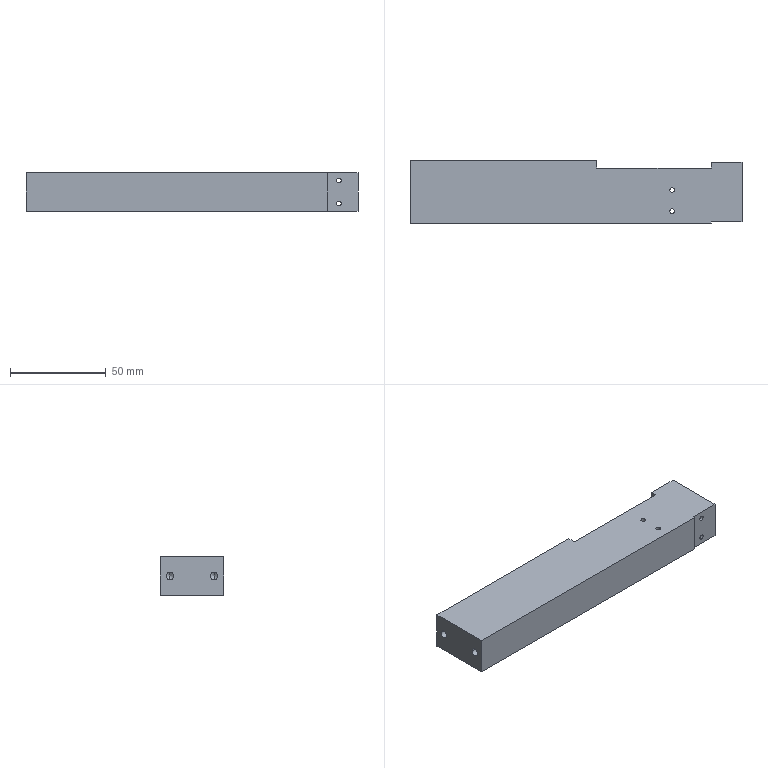Part | SolidWorks | features BaseBody 1 | 1 solid | 36 faces | box 173.5 x 33 x 20 mm | volume 108000 mm3 | cylinder 16 | plane 12 | cone 8 | commonest cylinder face diameters 2.459 x8 4.134 x8
STEP:
#1=CARTESIAN_POINT('',(21.865,283.98,0.));
#2=VERTEX_POINT('',#1);
#3=CARTESIAN_POINT('',(19.406,283.98,0.));
#4=VERTEX_POINT('',#3);
#5=CARTESIAN_POINT('',(20.636,283.98,0.));
#6=DIRECTION('',(0.,0.,-1.));
#7=DIRECTION('',(1.,0.,0.));
#8=AXIS2_PLACEMENT_3D('',#5,#6,#7);
#9=CIRCLE('',#8,1.23);
#10=EDGE_CURVE('',#2,#4,#9,.T.);
#11=ORIENTED_EDGE('',*,*,#10,.T.);
#12=CARTESIAN_POINT('',(19.406,283.98,20.));
#13=VERTEX_POINT('',#12);
#14=CARTESIAN_POINT('',(19.406,283.98,-157.739));
#15=DIRECTION('',(0.,0.,1.));
#16=VECTOR('',#15,1000.);
#17=LINE('',#14,#16);
#18=EDGE_CURVE('',#4,#13,#17,.T.);
#19=ORIENTED_EDGE('',*,*,#18,.T.);
#20=CARTESIAN_POINT('',(21.865,283.98,20.));
#21=VERTEX_POINT('',#20);
#22=CARTESIAN_POINT('',(20.636,283.98,20.));
#23=DIRECTION('',(0.,0.,-1.));
#24=DIRECTION('',(1.,0.,0.));
#25=AXIS2_PLACEMENT_3D('',#22,#23,#24);
#26=CIRCLE('',#25,1.23);
#27=EDGE_CURVE('',#21,#13,#26,.T.);
#28=ORIENTED_EDGE('',*,*,#27,.F.);
#29=CARTESIAN_POINT('',(21.865,283.98,-157.739));
#30=DIRECTION('',(0.,0.,1.));
#31=VECTOR('',#30,1000.);
#32=LINE('',#29,#31);
#33=EDGE_CURVE('',#2,#21,#32,.T.);
#34=ORIENTED_EDGE('',*,*,#33,.F.);
#35=EDGE_LOOP('',(#11,#19,#28,#34));
#36=FACE_OUTER_BOUND('',#35,.T.);
#37=CARTESIAN_POINT('',(20.636,283.98,-157.739));
#38=DIRECTION('',(0.,0.,1.));
#39=DIRECTION('',(1.,0.,0.));
#40=AXIS2_PLACEMENT_3D('',#37,#38,#39);
#41=CYLINDRICAL_SURFACE('',#40,1.23);
#42=ADVANCED_FACE('',(#36),#41,.F.);
#43=CARTESIAN_POINT('',(21.865,272.98,0.));
#44=VERTEX_POINT('',#43);
#45=CARTESIAN_POINT('',(19.406,272.98,0.));
#46=VERTEX_POINT('',#45);
#47=CARTESIAN_POINT('',(20.636,272.98,0.));
#48=DIRECTION('',(0.,0.,-1.));
#49=DIRECTION('',(1.,0.,0.));
#50=AXIS2_PLACEMENT_3D('',#47,#48,#49);
#51=CIRCLE('',#50,1.23);
#52=EDGE_CURVE('',#44,#46,#51,.T.);
#53=ORIENTED_EDGE('',*,*,#52,.T.);
#54=CARTESIAN_POINT('',(19.406,272.98,20.));
#55=VERTEX_POINT('',#54);
#56=CARTESIAN_POINT('',(19.406,272.98,-157.739));
#57=DIRECTION('',(0.,0.,1.));
#58=VECTOR('',#57,1000.);
#59=LINE('',#56,#58);
#60=EDGE_CURVE('',#46,#55,#59,.T.);
#61=ORIENTED_EDGE('',*,*,#60,.T.);
#62=CARTESIAN_POINT('',(21.865,272.98,20.));
#63=VERTEX_POINT('',#62);
#64=CARTESIAN_POINT('',(20.636,272.98,20.));
#65=DIRECTION('',(0.,0.,-1.));
#66=DIRECTION('',(1.,0.,0.));
#67=AXIS2_PLACEMENT_3D('',#64,#65,#66);
#68=CIRCLE('',#67,1.23);
#69=EDGE_CURVE('',#63,#55,#68,.T.);
#70=ORIENTED_EDGE('',*,*,#69,.F.);
#71=CARTESIAN_POINT('',(21.865,272.98,-157.739));
#72=DIRECTION('',(0.,0.,1.));
#73=VECTOR('',#72,1000.);
#74=LINE('',#71,#73);
#75=EDGE_CURVE('',#44,#63,#74,.T.);
#76=ORIENTED_EDGE('',*,*,#75,.F.);
#77=EDGE_LOOP('',(#53,#61,#70,#76));
#78=FACE_OUTER_BOUND('',#77,.T.);
#79=CARTESIAN_POINT('',(20.636,272.98,-157.739));
#80=DIRECTION('',(0.,0.,1.));
#81=DIRECTION('',(1.,0.,0.));
#82=AXIS2_PLACEMENT_3D('',#79,#80,#81);
#83=CYLINDRICAL_SURFACE('',#82,1.23);
#84=ADVANCED_FACE('',(#78),#83,.F.);
#85=CARTESIAN_POINT('',(-1.797,289.48,10.));
#86=VERTEX_POINT('',#85);
#87=CARTESIAN_POINT('',(-3.864,289.48,7.933));
#88=VERTEX_POINT('',#87);
#89=CARTESIAN_POINT('',(-3.864,289.48,10.));
#90=DIRECTION('',(0.,1.,0.));
#91=DIRECTION('',(-1.,0.,0.));
#92=AXIS2_PLACEMENT_3D('',#89,#90,#91);
#93=CIRCLE('',#92,2.067);
#94=EDGE_CURVE('',#86,#88,#93,.T.);
#95=ORIENTED_EDGE('',*,*,#94,.F.);
#96=CARTESIAN_POINT('',(-1.797,295.48,10.));
#97=VERTEX_POINT('',#96);
#98=CARTESIAN_POINT('',(-1.797,294.48,10.));
#99=DIRECTION('',(0.,1.,0.));
#100=VECTOR('',#99,1000.);
#101=LINE('',#98,#100);
#102=EDGE_CURVE('',#86,#97,#101,.T.);
#103=ORIENTED_EDGE('',*,*,#102,.T.);
#104=CARTESIAN_POINT('',(-5.931,295.48,10.));
#105=VERTEX_POINT('',#104);
#106=CARTESIAN_POINT('',(-3.864,295.48,10.));
#107=DIRECTION('',(0.,-1.,0.));
#108=DIRECTION('',(-1.,0.,0.));
#109=AXIS2_PLACEMENT_3D('',#106,#107,#108);
#110=CIRCLE('',#109,2.067);
#111=EDGE_CURVE('',#105,#97,#110,.T.);
#112=ORIENTED_EDGE('',*,*,#111,.F.);
#113=CARTESIAN_POINT('',(-5.931,289.48,10.));
#114=VERTEX_POINT('',#113);
#115=CARTESIAN_POINT('',(-5.931,294.48,10.));
#116=DIRECTION('',(0.,1.,0.));
#117=VECTOR('',#116,1000.);
#118=LINE('',#115,#117);
#119=EDGE_CURVE('',#114,#105,#118,.T.);
#120=ORIENTED_EDGE('',*,*,#119,.F.);
#121=CARTESIAN_POINT('',(-3.864,289.48,10.));
#122=DIRECTION('',(0.,1.,0.));
#123=DIRECTION('',(-1.,0.,0.));
#124=AXIS2_PLACEMENT_3D('',#121,#122,#123);
#125=CIRCLE('',#124,2.067);
#126=EDGE_CURVE('',#88,#114,#125,.T.);
#127=ORIENTED_EDGE('',*,*,#126,.F.);
#128=EDGE_LOOP('',(#95,#103,#112,#120,#127));
#129=FACE_OUTER_BOUND('',#128,.T.);
#130=CARTESIAN_POINT('',(-3.864,294.48,10.));
#131=DIRECTION('',(0.,1.,0.));
#132=DIRECTION('',(-1.,0.,0.));
#133=AXIS2_PLACEMENT_3D('',#130,#131,#132);
#134=CYLINDRICAL_SURFACE('',#133,2.067);
#135=ADVANCED_FACE('',(#129),#134,.F.);
#136=CARTESIAN_POINT('',(28.203,289.48,10.));
#137=VERTEX_POINT('',#136);
#138=CARTESIAN_POINT('',(26.136,289.48,7.933));
#139=VERTEX_POINT('',#138);
#140=CARTESIAN_POINT('',(26.136,289.48,10.));
#141=DIRECTION('',(0.,1.,0.));
#142=DIRECTION('',(-1.,0.,0.));
#143=AXIS2_PLACEMENT_3D('',#140,#141,#142);
#144=CIRCLE('',#143,2.067);
#145=EDGE_CURVE('',#137,#139,#144,.T.);
#146=ORIENTED_EDGE('',*,*,#145,.F.);
#147=CARTESIAN_POINT('',(28.203,295.48,10.));
#148=VERTEX_POINT('',#147);
#149=CARTESIAN_POINT('',(28.203,294.48,10.));
#150=DIRECTION('',(0.,1.,0.));
#151=VECTOR('',#150,1000.);
#152=LINE('',#149,#151);
#153=EDGE_CURVE('',#137,#148,#152,.T.);
#154=ORIENTED_EDGE('',*,*,#153,.T.);
#155=CARTESIAN_POINT('',(24.069,295.48,10.));
#156=VERTEX_POINT('',#155);
#157=CARTESIAN_POINT('',(26.136,295.48,10.));
#158=DIRECTION('',(0.,-1.,0.));
#159=DIRECTION('',(-1.,0.,0.));
#160=AXIS2_PLACEMENT_3D('',#157,#158,#159);
#161=CIRCLE('',#160,2.067);
#162=EDGE_CURVE('',#156,#148,#161,.T.);
#163=ORIENTED_EDGE('',*,*,#162,.F.);
#164=CARTESIAN_POINT('',(24.069,289.48,10.));
#165=VERTEX_POINT('',#164);
#166=CARTESIAN_POINT('',(24.069,294.48,10.));
#167=DIRECTION('',(0.,1.,0.));
#168=VECTOR('',#167,1000.);
#169=LINE('',#166,#168);
#170=EDGE_CURVE('',#165,#156,#169,.T.);
#171=ORIENTED_EDGE('',*,*,#170,.F.);
#172=CARTESIAN_POINT('',(26.136,289.48,10.));
#173=DIRECTION('',(0.,1.,0.));
#174=DIRECTION('',(-1.,0.,0.));
#175=AXIS2_PLACEMENT_3D('',#172,#173,#174);
#176=CIRCLE('',#175,2.067);
#177=EDGE_CURVE('',#139,#165,#176,.T.);
#178=ORIENTED_EDGE('',*,*,#177,.F.);
#179=EDGE_LOOP('',(#146,#154,#163,#171,#178));
#180=FACE_OUTER_BOUND('',#179,.T.);
#181=CARTESIAN_POINT('',(26.136,294.48,10.));
#182=DIRECTION('',(0.,1.,0.));
#183=DIRECTION('',(-1.,0.,0.));
#184=AXIS2_PLACEMENT_3D('',#181,#182,#183);
#185=CYLINDRICAL_SURFACE('',#184,2.067);
#186=ADVANCED_FACE('',(#180),#185,.F.);
#187=CARTESIAN_POINT('',(45.906,267.48,16.));
#188=VERTEX_POINT('',#187);
#189=CARTESIAN_POINT('',(48.365,267.48,16.));
#190=VERTEX_POINT('',#189);
#191=CARTESIAN_POINT('',(47.136,267.48,16.));
#192=DIRECTION('',(0.,-1.,0.));
#193=DIRECTION('',(-1.,0.,0.));
#194=AXIS2_PLACEMENT_3D('',#191,#192,#193);
#195=CIRCLE('',#194,1.23);
#196=EDGE_CURVE('',#188,#190,#195,.T.);
#197=ORIENTED_EDGE('',*,*,#196,.T.);
#198=CARTESIAN_POINT('',(48.365,298.48,16.));
#199=VERTEX_POINT('',#198);
#200=CARTESIAN_POINT('',(48.365,121.741,16.));
#201=DIRECTION('',(0.,1.,0.));
#202=VECTOR('',#201,1000.);
#203=LINE('',#200,#202);
#204=EDGE_CURVE('',#190,#199,#203,.T.);
#205=ORIENTED_EDGE('',*,*,#204,.T.);
#206=CARTESIAN_POINT('',(45.906,298.48,16.));
#207=VERTEX_POINT('',#206);
#208=CARTESIAN_POINT('',(47.136,298.48,16.));
#209=DIRECTION('',(0.,-1.,0.));
#210=DIRECTION('',(-1.,0.,0.));
#211=AXIS2_PLACEMENT_3D('',#208,#209,#210);
#212=CIRCLE('',#211,1.23);
#213=EDGE_CURVE('',#207,#199,#212,.T.);
#214=ORIENTED_EDGE('',*,*,#213,.F.);
#215=CARTESIAN_POINT('',(45.906,121.741,16.));
#216=DIRECTION('',(0.,1.,0.));
#217=VECTOR('',#216,1000.);
#218=LINE('',#215,#217);
#219=EDGE_CURVE('',#188,#207,#218,.T.);
#220=ORIENTED_EDGE('',*,*,#219,.F.);
#221=EDGE_LOOP('',(#197,#205,#214,#220));
#222=FACE_OUTER_BOUND('',#221,.T.);
#223=CARTESIAN_POINT('',(47.136,121.741,16.));
#224=DIRECTION('',(0.,1.,0.));
#225=DIRECTION('',(-1.,0.,0.));
#226=AXIS2_PLACEMENT_3D('',#223,#224,#225);
#227=CYLINDRICAL_SURFACE('',#226,1.23);
#228=ADVANCED_FACE('',(#222),#227,.F.);
#229=CARTESIAN_POINT('',(45.906,267.48,4.));
#230=VERTEX_POINT('',#229);
#231=CARTESIAN_POINT('',(48.365,267.48,4.));
#232=VERTEX_POINT('',#231);
#233=CARTESIAN_POINT('',(47.136,267.48,4.));
#234=DIRECTION('',(0.,-1.,0.));
#235=DIRECTION('',(-1.,0.,0.));
#236=AXIS2_PLACEMENT_3D('',#233,#234,#235);
#237=CIRCLE('',#236,1.23);
#238=EDGE_CURVE('',#230,#232,#237,.T.);
#239=ORIENTED_EDGE('',*,*,#238,.T.);
#240=CARTESIAN_POINT('',(48.365,298.48,4.));
#241=VERTEX_POINT('',#240);
#242=CARTESIAN_POINT('',(48.365,121.741,4.));
#243=DIRECTION('',(0.,1.,0.));
#244=VECTOR('',#243,1000.);
#245=LINE('',#242,#244);
#246=EDGE_CURVE('',#232,#241,#245,.T.);
#247=ORIENTED_EDGE('',*,*,#246,.T.);
#248=CARTESIAN_POINT('',(45.906,298.48,4.));
#249=VERTEX_POINT('',#248);
#250=CARTESIAN_POINT('',(47.136,298.48,4.));
#251=DIRECTION('',(0.,-1.,0.));
#252=DIRECTION('',(-1.,0.,0.));
#253=AXIS2_PLACEMENT_3D('',#250,#251,#252);
#254=CIRCLE('',#253,1.23);
#255=EDGE_CURVE('',#249,#241,#254,.T.);
#256=ORIENTED_EDGE('',*,*,#255,.F.);
#257=CARTESIAN_POINT('',(45.906,121.741,4.));
#258=DIRECTION('',(0.,1.,0.));
#259=VECTOR('',#258,1000.);
#260=LINE('',#257,#259);
#261=EDGE_CURVE('',#230,#249,#260,.T.);
#262=ORIENTED_EDGE('',*,*,#261,.F.);
#263=EDGE_LOOP('',(#239,#247,#256,#262));
#264=FACE_OUTER_BOUND('',#263,.T.);
#265=CARTESIAN_POINT('',(47.136,121.741,4.));
#266=DIRECTION('',(0.,1.,0.));
#267=DIRECTION('',(-1.,0.,0.));
#268=AXIS2_PLACEMENT_3D('',#265,#266,#267);
#269=CYLINDRICAL_SURFACE('',#268,1.23);
#270=ADVANCED_FACE('',(#264),#269,.F.);
#271=CARTESIAN_POINT('',(-101.364,296.547,10.));
#272=VERTEX_POINT('',#271);
#273=CARTESIAN_POINT('',(-101.364,294.48,7.933));
#274=VERTEX_POINT('',#273);
#275=CARTESIAN_POINT('',(-101.364,294.48,10.));
#276=DIRECTION('',(-1.,0.,0.));
#277=DIRECTION('',(0.,-1.,0.));
#278=AXIS2_PLACEMENT_3D('',#275,#276,#277);
#279=CIRCLE('',#278,2.067);
#280=EDGE_CURVE('',#272,#274,#279,.T.);
#281=ORIENTED_EDGE('',*,*,#280,.F.);
#282=CARTESIAN_POINT('',(-116.364,296.547,10.));
#283=VERTEX_POINT('',#282);
#284=CARTESIAN_POINT('',(-108.864,296.547,10.));
#285=DIRECTION('',(-1.,0.,0.));
#286=VECTOR('',#285,1000.);
#287=LINE('',#284,#286);
#288=EDGE_CURVE('',#272,#283,#287,.T.);
#289=ORIENTED_EDGE('',*,*,#288,.T.);
#290=CARTESIAN_POINT('',(-116.364,292.413,10.));
#291=VERTEX_POINT('',#290);
#292=CARTESIAN_POINT('',(-116.364,294.48,10.));
#293=DIRECTION('',(1.,0.,0.));
#294=DIRECTION('',(0.,-1.,0.));
#295=AXIS2_PLACEMENT_3D('',#292,#293,#294);
#296=CIRCLE('',#295,2.067);
#297=EDGE_CURVE('',#291,#283,#296,.T.);
#298=ORIENTED_EDGE('',*,*,#297,.F.);
#299=CARTESIAN_POINT('',(-101.364,292.413,10.));
#300=VERTEX_POINT('',#299);
#301=CARTESIAN_POINT('',(-108.864,292.413,10.));
#302=DIRECTION('',(-1.,0.,0.));
#303=VECTOR('',#302,1000.);
#304=LINE('',#301,#303);
#305=EDGE_CURVE('',#300,#291,#304,.T.);
#306=ORIENTED_EDGE('',*,*,#305,.F.);
#307=CARTESIAN_POINT('',(-101.364,294.48,10.));
#308=DIRECTION('',(-1.,0.,0.));
#309=DIRECTION('',(0.,-1.,0.));
#310=AXIS2_PLACEMENT_3D('',#307,#308,#309);
#311=CIRCLE('',#310,2.067);
#312=EDGE_CURVE('',#274,#300,#311,.T.);
#313=ORIENTED_EDGE('',*,*,#312,.F.);
#314=EDGE_LOOP('',(#281,#289,#298,#306,#313));
#315=FACE_OUTER_BOUND('',#314,.T.);
#316=CARTESIAN_POINT('',(-108.864,294.48,10.));
#317=DIRECTION('',(-1.,0.,0.));
#318=DIRECTION('',(0.,-1.,0.));
#319=AXIS2_PLACEMENT_3D('',#316,#317,#318);
#320=CYLINDRICAL_SURFACE('',#319,2.067);
#321=ADVANCED_FACE('',(#315),#320,.F.);
#322=CARTESIAN_POINT('',(-101.364,273.547,10.));
#323=VERTEX_POINT('',#322);
#324=CARTESIAN_POINT('',(-101.364,271.48,7.933));
#325=VERTEX_POINT('',#324);
#326=CARTESIAN_POINT('',(-101.364,271.48,10.));
#327=DIRECTION('',(-1.,0.,0.));
#328=DIRECTION('',(0.,-1.,0.));
#329=AXIS2_PLACEMENT_3D('',#326,#327,#328);
#330=CIRCLE('',#329,2.067);
#331=EDGE_CURVE('',#323,#325,#330,.T.);
#332=ORIENTED_EDGE('',*,*,#331,.F.);
#333=CARTESIAN_POINT('',(-116.364,273.547,10.));
#334=VERTEX_POINT('',#333);
#335=CARTESIAN_POINT('',(-108.864,273.547,10.));
#336=DIRECTION('',(-1.,0.,0.));
#337=VECTOR('',#336,1000.);
#338=LINE('',#335,#337);
#339=EDGE_CURVE('',#323,#334,#338,.T.);
#340=ORIENTED_EDGE('',*,*,#339,.T.);
#341=CARTESIAN_POINT('',(-116.364,269.413,10.));
#342=VERTEX_POINT('',#341);
#343=CARTESIAN_POINT('',(-116.364,271.48,10.));
#344=DIRECTION('',(1.,0.,0.));
#345=DIRECTION('',(0.,-1.,0.));
#346=AXIS2_PLACEMENT_3D('',#343,#344,#345);
#347=CIRCLE('',#346,2.067);
#348=EDGE_CURVE('',#342,#334,#347,.T.);
#349=ORIENTED_EDGE('',*,*,#348,.F.);
#350=CARTESIAN_POINT('',(-101.364,269.413,10.));
#351=VERTEX_POINT('',#350);
#352=CARTESIAN_POINT('',(-108.864,269.413,10.));
#353=DIRECTION('',(-1.,0.,0.));
#354=VECTOR('',#353,1000.);
#355=LINE('',#352,#354);
#356=EDGE_CURVE('',#351,#342,#355,.T.);
#357=ORIENTED_EDGE('',*,*,#356,.F.);
#358=CARTESIAN_POINT('',(-101.364,271.48,10.));
#359=DIRECTION('',(-1.,0.,0.));
#360=DIRECTION('',(0.,-1.,0.));
#361=AXIS2_PLACEMENT_3D('',#358,#359,#360);
#362=CIRCLE('',#361,2.067);
#363=EDGE_CURVE('',#325,#351,#362,.T.);
#364=ORIENTED_EDGE('',*,*,#363,.F.);
#365=EDGE_LOOP('',(#332,#340,#349,#357,#364));
#366=FACE_OUTER_BOUND('',#365,.T.);
#367=CARTESIAN_POINT('',(-108.864,271.48,10.));
#368=DIRECTION('',(-1.,0.,0.));
#369=DIRECTION('',(0.,-1.,0.));
#370=AXIS2_PLACEMENT_3D('',#367,#368,#369);
#371=CYLINDRICAL_SURFACE('',#370,2.067);
#372=ADVANCED_FACE('',(#366),#371,.F.);
#373=CARTESIAN_POINT('',(-3.864,288.238,10.));
#374=VERTEX_POINT('',#373);
#375=CARTESIAN_POINT('',(-3.864,289.48,12.067));
#376=VERTEX_POINT('',#375);
#377=CARTESIAN_POINT('',(-3.864,289.48,12.067));
#378=DIRECTION('',(0.,0.515,0.8572));
#379=VECTOR('',#378,1000.);
#380=LINE('',#377,#379);
#381=EDGE_CURVE('',#374,#376,#380,.T.);
#382=ORIENTED_EDGE('',*,*,#381,.F.);
#383=CARTESIAN_POINT('',(-3.864,289.48,7.933));
#384=DIRECTION('',(0.,0.515,-0.8572));
#385=VECTOR('',#384,1000.);
#386=LINE('',#383,#385);
#387=EDGE_CURVE('',#374,#88,#386,.T.);
#388=ORIENTED_EDGE('',*,*,#387,.T.);
#389=ORIENTED_EDGE('',*,*,#126,.T.);
#390=CARTESIAN_POINT('',(-3.864,289.48,10.));
#391=DIRECTION('',(0.,1.,0.));
#392=DIRECTION('',(-1.,0.,0.));
#393=AXIS2_PLACEMENT_3D('',#390,#391,#392);
#394=CIRCLE('',#393,2.067);
#395=EDGE_CURVE('',#114,#376,#394,.T.);
#396=ORIENTED_EDGE('',*,*,#395,.T.);
#397=EDGE_LOOP('',(#382,#388,#389,#396));
#398=FACE_OUTER_BOUND('',#397,.T.);
#399=CARTESIAN_POINT('',(-3.864,289.48,10.));
#400=DIRECTION('',(0.,1.,0.));
#401=DIRECTION('',(0.,0.,1.));
#402=AXIS2_PLACEMENT_3D('',#399,#400,#401);
#403=CONICAL_SURFACE('',#402,2.067,1.03);
#404=ADVANCED_FACE('',(#398),#403,.F.);
#405=CARTESIAN_POINT('',(26.136,288.238,10.));
#406=VERTEX_POINT('',#405);
#407=CARTESIAN_POINT('',(26.136,289.48,12.067));
#408=VERTEX_POINT('',#407);
#409=CARTESIAN_POINT('',(26.136,289.48,12.067));
#410=DIRECTION('',(0.,0.515,0.8572));
#411=VECTOR('',#410,1000.);
#412=LINE('',#409,#411);
#413=EDGE_CURVE('',#406,#408,#412,.T.);
#414=ORIENTED_EDGE('',*,*,#413,.F.);
#415=CARTESIAN_POINT('',(26.136,289.48,7.933));
#416=DIRECTION('',(0.,0.515,-0.8572));
#417=VECTOR('',#416,1000.);
#418=LINE('',#415,#417);
#419=EDGE_CURVE('',#406,#139,#418,.T.);
#420=ORIENTED_EDGE('',*,*,#419,.T.);
#421=ORIENTED_EDGE('',*,*,#177,.T.);
#422=CARTESIAN_POINT('',(26.136,289.48,10.));
#423=DIRECTION('',(0.,1.,0.));
#424=DIRECTION('',(-1.,0.,0.));
#425=AXIS2_PLACEMENT_3D('',#422,#423,#424);
#426=CIRCLE('',#425,2.067);
#427=EDGE_CURVE('',#165,#408,#426,.T.);
#428=ORIENTED_EDGE('',*,*,#427,.T.);
#429=EDGE_LOOP('',(#414,#420,#421,#428));
#430=FACE_OUTER_BOUND('',#429,.T.);
#431=CARTESIAN_POINT('',(26.136,289.48,10.));
#432=DIRECTION('',(0.,1.,0.));
#433=DIRECTION('',(0.,0.,1.));
#434=AXIS2_PLACEMENT_3D('',#431,#432,#433);
#435=CONICAL_SURFACE('',#434,2.067,1.03);
#436=ADVANCED_FACE('',(#430),#435,.F.);
#437=CARTESIAN_POINT('',(-100.122,294.48,10.));
#438=VERTEX_POINT('',#437);
#439=CARTESIAN_POINT('',(-101.364,294.48,12.067));
#440=VERTEX_POINT('',#439);
#441=CARTESIAN_POINT('',(-101.364,294.48,12.067));
#442=DIRECTION('',(-0.515,0.,0.8572));
#443=VECTOR('',#442,1000.);
#444=LINE('',#441,#443);
#445=EDGE_CURVE('',#438,#440,#444,.T.);
#446=ORIENTED_EDGE('',*,*,#445,.F.);
#447=CARTESIAN_POINT('',(-101.364,294.48,7.933));
#448=DIRECTION('',(-0.515,0.,-0.8572));
#449=VECTOR('',#448,1000.);
#450=LINE('',#447,#449);
#451=EDGE_CURVE('',#438,#274,#450,.T.);
#452=ORIENTED_EDGE('',*,*,#451,.T.);
#453=ORIENTED_EDGE('',*,*,#312,.T.);
#454=CARTESIAN_POINT('',(-101.364,294.48,10.));
#455=DIRECTION('',(-1.,0.,0.));
#456=DIRECTION('',(0.,-1.,0.));
#457=AXIS2_PLACEMENT_3D('',#454,#455,#456);
#458=CIRCLE('',#457,2.067);
#459=EDGE_CURVE('',#300,#440,#458,.T.);
#460=ORIENTED_EDGE('',*,*,#459,.T.);
#461=EDGE_LOOP('',(#446,#452,#453,#460));
#462=FACE_OUTER_BOUND('',#461,.T.);
#463=CARTESIAN_POINT('',(-101.364,294.48,10.));
#464=DIRECTION('',(-1.,0.,0.));
#465=DIRECTION('',(0.,0.,1.));
#466=AXIS2_PLACEMENT_3D('',#463,#464,#465);
#467=CONICAL_SURFACE('',#466,2.067,1.03);
#468=ADVANCED_FACE('',(#462),#467,.F.);
#469=CARTESIAN_POINT('',(-100.122,271.48,10.));
#470=VERTEX_POINT('',#469);
#471=CARTESIAN_POINT('',(-101.364,271.48,12.067));
#472=VERTEX_POINT('',#471);
#473=CARTESIAN_POINT('',(-101.364,271.48,12.067));
#474=DIRECTION('',(-0.515,0.,0.8572));
#475=VECTOR('',#474,1000.);
#476=LINE('',#473,#475);
#477=EDGE_CURVE('',#470,#472,#476,.T.);
#478=ORIENTED_EDGE('',*,*,#477,.F.);
#479=CARTESIAN_POINT('',(-101.364,271.48,7.933));
#480=DIRECTION('',(-0.515,0.,-0.8572));
#481=VECTOR('',#480,1000.);
#482=LINE('',#479,#481);
#483=EDGE_CURVE('',#470,#325,#482,.T.);
#484=ORIENTED_EDGE('',*,*,#483,.T.);
#485=ORIENTED_EDGE('',*,*,#363,.T.);
#486=CARTESIAN_POINT('',(-101.364,271.48,10.));
#487=DIRECTION('',(-1.,0.,0.));
#488=DIRECTION('',(0.,-1.,0.));
#489=AXIS2_PLACEMENT_3D('',#486,#487,#488);
#490=CIRCLE('',#489,2.067);
#491=EDGE_CURVE('',#351,#472,#490,.T.);
#492=ORIENTED_EDGE('',*,*,#491,.T.);
#493=EDGE_LOOP('',(#478,#484,#485,#492));
#494=FACE_OUTER_BOUND('',#493,.T.);
#495=CARTESIAN_POINT('',(-101.364,271.48,10.));
#496=DIRECTION('',(-1.,0.,0.));
#497=DIRECTION('',(0.,0.,1.));
#498=AXIS2_PLACEMENT_3D('',#495,#496,#497);
#499=CONICAL_SURFACE('',#498,2.067,1.03);
#500=ADVANCED_FACE('',(#494),#499,.F.);
#501=ORIENTED_EDGE('',*,*,#10,.F.);
#502=CARTESIAN_POINT('',(20.636,283.98,0.));
#503=DIRECTION('',(0.,0.,-1.));
#504=DIRECTION('',(1.,0.,0.));
#505=AXIS2_PLACEMENT_3D('',#502,#503,#504);
#506=CIRCLE('',#505,1.23);
#507=EDGE_CURVE('',#4,#2,#506,.T.);
#508=ORIENTED_EDGE('',*,*,#507,.F.);
#509=EDGE_LOOP('',(#501,#508));
#510=FACE_BOUND('',#509,.T.);
#511=ORIENTED_EDGE('',*,*,#52,.F.);
#512=CARTESIAN_POINT('',(20.636,272.98,0.));
#513=DIRECTION('',(0.,0.,-1.));
#514=DIRECTION('',(1.,0.,0.));
#515=AXIS2_PLACEMENT_3D('',#512,#513,#514);
#516=CIRCLE('',#515,1.23);
#517=EDGE_CURVE('',#46,#44,#516,.T.);
#518=ORIENTED_EDGE('',*,*,#517,.F.);
#519=EDGE_LOOP('',(#511,#518));
#520=FACE_BOUND('',#519,.T.);
#521=CARTESIAN_POINT('',(41.136,295.48,0.));
#522=VERTEX_POINT('',#521);
#523=CARTESIAN_POINT('',(-18.864,295.48,0.));
#524=VERTEX_POINT('',#523);
#525=CARTESIAN_POINT('',(-29.614,295.48,0.));
#526=DIRECTION('',(-1.,0.,0.));
#527=VECTOR('',#526,1000.);
#528=LINE('',#525,#527);
#529=EDGE_CURVE('',#522,#524,#528,.T.);
#530=ORIENTED_EDGE('',*,*,#529,.F.);
#531=CARTESIAN_POINT('',(41.136,298.48,0.));
#532=VERTEX_POINT('',#531);
#533=CARTESIAN_POINT('',(41.136,282.98,0.));
#534=DIRECTION('',(0.,-1.,0.));
#535=VECTOR('',#534,1000.);
#536=LINE('',#533,#535);
#537=EDGE_CURVE('',#532,#522,#536,.T.);
#538=ORIENTED_EDGE('',*,*,#537,.F.);
#539=CARTESIAN_POINT('',(57.136,298.48,0.));
#540=VERTEX_POINT('',#539);
#541=CARTESIAN_POINT('',(-29.614,298.48,0.));
#542=DIRECTION('',(-1.,0.,0.));
#543=VECTOR('',#542,1000.);
#544=LINE('',#541,#543);
#545=EDGE_CURVE('',#540,#532,#544,.T.);
#546=ORIENTED_EDGE('',*,*,#545,.F.);
#547=CARTESIAN_POINT('',(57.136,267.48,0.));
#548=VERTEX_POINT('',#547);
#549=CARTESIAN_POINT('',(57.136,282.98,0.));
#550=DIRECTION('',(0.,1.,0.));
#551=VECTOR('',#550,1000.);
#552=LINE('',#549,#551);
#553=EDGE_CURVE('',#548,#540,#552,.T.);
#554=ORIENTED_EDGE('',*,*,#553,.F.);
#555=CARTESIAN_POINT('',(41.136,267.48,0.));
#556=VERTEX_POINT('',#555);
#557=CARTESIAN_POINT('',(-29.614,267.48,0.));
#558=DIRECTION('',(1.,0.,0.));
#559=VECTOR('',#558,1000.);
#560=LINE('',#557,#559);
#561=EDGE_CURVE('',#556,#548,#560,.T.);
#562=ORIENTED_EDGE('',*,*,#561,.F.);
#563=CARTESIAN_POINT('',(41.136,266.48,0.));
#564=VERTEX_POINT('',#563);
#565=CARTESIAN_POINT('',(41.136,266.48,0.));
#566=DIRECTION('',(0.,-1.,0.));
#567=VECTOR('',#566,1000.);
#568=LINE('',#565,#567);
#569=EDGE_CURVE('',#556,#564,#568,.T.);
#570=ORIENTED_EDGE('',*,*,#569,.T.);
#571=CARTESIAN_POINT('',(-116.364,266.48,0.));
#572=VERTEX_POINT('',#571);
#573=CARTESIAN_POINT('',(-29.614,266.48,0.));
#574=DIRECTION('',(1.,0.,0.));
#575=VECTOR('',#574,1000.);
#576=LINE('',#573,#575);
#577=EDGE_CURVE('',#572,#564,#576,.T.);
#578=ORIENTED_EDGE('',*,*,#577,.F.);
#579=CARTESIAN_POINT('',(-116.364,299.48,0.));
#580=VERTEX_POINT('',#579);
#581=CARTESIAN_POINT('',(-116.364,282.98,0.));
#582=DIRECTION('',(0.,-1.,0.));
#583=VECTOR('',#582,1000.);
#584=LINE('',#581,#583);
#585=EDGE_CURVE('',#580,#572,#584,.T.);
#586=ORIENTED_EDGE('',*,*,#585,.F.);
#587=CARTESIAN_POINT('',(-18.864,299.48,0.));
#588=VERTEX_POINT('',#587);
#589=CARTESIAN_POINT('',(-29.614,299.48,0.));
#590=DIRECTION('',(-1.,0.,0.));
#591=VECTOR('',#590,1000.);
#592=LINE('',#589,#591);
#593=EDGE_CURVE('',#588,#580,#592,.T.);
#594=ORIENTED_EDGE('',*,*,#593,.F.);
#595=CARTESIAN_POINT('',(-18.864,282.98,0.));
#596=DIRECTION('',(0.,1.,0.));
#597=VECTOR('',#596,1000.);
#598=LINE('',#595,#597);
#599=EDGE_CURVE('',#524,#588,#598,.T.);
#600=ORIENTED_EDGE('',*,*,#599,.F.);
#601=EDGE_LOOP('',(#530,#538,#546,#554,#562,#570,#578,#586,#594,#600));
#602=FACE_OUTER_BOUND('',#601,.T.);
#603=CARTESIAN_POINT('',(-29.614,282.98,0.));
#604=DIRECTION('',(0.,0.,1.));
#605=DIRECTION('',(1.,0.,0.));
#606=AXIS2_PLACEMENT_3D('',#603,#604,#605);
#607=PLANE('',#606);
#608=ADVANCED_FACE('',(#510,#520,#602),#607,.F.);
#609=ORIENTED_EDGE('',*,*,#18,.F.);
#610=ORIENTED_EDGE('',*,*,#507,.T.);
#611=ORIENTED_EDGE('',*,*,#33,.T.);
#612=CARTESIAN_POINT('',(20.636,283.98,20.));
#613=DIRECTION('',(0.,0.,-1.));
#614=DIRECTION('',(1.,0.,0.));
#615=AXIS2_PLACEMENT_3D('',#612,#613,#614);
#616=CIRCLE('',#615,1.23);
#617=EDGE_CURVE('',#13,#21,#616,.T.);
#618=ORIENTED_EDGE('',*,*,#617,.F.);
#619=EDGE_LOOP('',(#609,#610,#611,#618));
#620=FACE_OUTER_BOUND('',#619,.T.);
#621=CARTESIAN_POINT('',(20.636,283.98,-157.739));
#622=DIRECTION('',(0.,0.,1.));
#623=DIRECTION('',(1.,0.,0.));
#624=AXIS2_PLACEMENT_3D('',#621,#622,#623);
#625=CYLINDRICAL_SURFACE('',#624,1.23);
#626=ADVANCED_FACE('',(#620),#625,.F.);
#627=ORIENTED_EDGE('',*,*,#60,.F.);
#628=ORIENTED_EDGE('',*,*,#517,.T.);
#629=ORIENTED_EDGE('',*,*,#75,.T.);
#630=CARTESIAN_POINT('',(20.636,272.98,20.));
#631=DIRECTION('',(0.,0.,-1.));
#632=DIRECTION('',(1.,0.,0.));
#633=AXIS2_PLACEMENT_3D('',#630,#631,#632);
#634=CIRCLE('',#633,1.23);
#635=EDGE_CURVE('',#55,#63,#634,.T.);
#636=ORIENTED_EDGE('',*,*,#635,.F.);
#637=EDGE_LOOP('',(#627,#628,#629,#636));
#638=FACE_OUTER_BOUND('',#637,.T.);
#639=CARTESIAN_POINT('',(20.636,272.98,-157.739));
#640=DIRECTION('',(0.,0.,1.));
#641=DIRECTION('',(1.,0.,0.));
#642=AXIS2_PLACEMENT_3D('',#639,#640,#641);
#643=CYLINDRICAL_SURFACE('',#642,1.23);
#644=ADVANCED_FACE('',(#638),#643,.F.);
#645=ORIENTED_EDGE('',*,*,#599,.T.);
#646=CARTESIAN_POINT('',(-18.864,299.48,20.));
#647=VERTEX_POINT('',#646);
#648=CARTESIAN_POINT('',(-18.864,299.48,0.));
#649=DIRECTION('',(0.,0.,-1.));
#650=VECTOR('',#649,1000.);
#651=LINE('',#648,#650);
#652=EDGE_CURVE('',#647,#588,#651,.T.);
#653=ORIENTED_EDGE('',*,*,#652,.F.);
#654=CARTESIAN_POINT('',(-18.864,295.48,20.));
#655=VERTEX_POINT('',#654);
#656=CARTESIAN_POINT('',(-18.864,299.48,20.));
#657=DIRECTION('',(0.,1.,0.));
#658=VECTOR('',#657,1000.);
#659=LINE('',#656,#658);
#660=EDGE_CURVE('',#655,#647,#659,.T.);
#661=ORIENTED_EDGE('',*,*,#660,.F.);
#662=CARTESIAN_POINT('',(-18.864,295.48,0.));
#663=DIRECTION('',(0.,0.,1.));
#664=VECTOR('',#663,1000.);
#665=LINE('',#662,#664);
#666=EDGE_CURVE('',#524,#655,#665,.T.);
#667=ORIENTED_EDGE('',*,*,#666,.F.);
#668=EDGE_LOOP('',(#645,#653,#661,#667));
#669=FACE_OUTER_BOUND('',#668,.T.);
#670=CARTESIAN_POINT('',(-18.864,299.48,0.));
#671=DIRECTION('',(-1.,0.,0.));
#672=DIRECTION('',(0.,0.,1.));
#673=AXIS2_PLACEMENT_3D('',#670,#671,#672);
#674=PLANE('',#673);
#675=ADVANCED_FACE('',(#669),#674,.F.);
#676=ORIENTED_EDGE('',*,*,#111,.T.);
#677=CARTESIAN_POINT('',(-3.864,295.48,10.));
#678=DIRECTION('',(0.,-1.,0.));
#679=DIRECTION('',(-1.,0.,0.));
#680=AXIS2_PLACEMENT_3D('',#677,#678,#679);
#681=CIRCLE('',#680,2.067);
#682=EDGE_CURVE('',#97,#105,#681,.T.);
#683=ORIENTED_EDGE('',*,*,#682,.T.);
#684=EDGE_LOOP('',(#676,#683));
#685=FACE_BOUND('',#684,.T.);
#686=ORIENTED_EDGE('',*,*,#162,.T.);
#687=CARTESIAN_POINT('',(26.136,295.48,10.));
#688=DIRECTION('',(0.,-1.,0.));
#689=DIRECTION('',(-1.,0.,0.));
#690=AXIS2_PLACEMENT_3D('',#687,#688,#689);
#691=CIRCLE('',#690,2.067);
#692=EDGE_CURVE('',#148,#156,#691,.T.);
#693=ORIENTED_EDGE('',*,*,#692,.T.);
#694=EDGE_LOOP('',(#686,#693));
#695=FACE_BOUND('',#694,.T.);
#696=CARTESIAN_POINT('',(41.136,295.48,20.));
#697=VERTEX_POINT('',#696);
#698=CARTESIAN_POINT('',(41.136,295.48,10.));
#699=DIRECTION('',(0.,0.,-1.));
#700=VECTOR('',#699,1000.);
#701=LINE('',#698,#700);
#702=EDGE_CURVE('',#697,#522,#701,.T.);
#703=ORIENTED_EDGE('',*,*,#702,.T.);
#704=ORIENTED_EDGE('',*,*,#529,.T.);
#705=ORIENTED_EDGE('',*,*,#666,.T.);
#706=CARTESIAN_POINT('',(11.136,295.48,20.));
#707=DIRECTION('',(1.,0.,0.));
#708=VECTOR('',#707,1000.);
#709=LINE('',#706,#708);
#710=EDGE_CURVE('',#655,#697,#709,.T.);
#711=ORIENTED_EDGE('',*,*,#710,.T.);
#712=EDGE_LOOP('',(#703,#704,#705,#711));
#713=FACE_OUTER_BOUND('',#712,.T.);
#714=CARTESIAN_POINT('',(11.136,295.48,10.));
#715=DIRECTION('',(0.,1.,0.));
#716=DIRECTION('',(0.,0.,1.));
#717=AXIS2_PLACEMENT_3D('',#714,#715,#716);
#718=PLANE('',#717);
#719=ADVANCED_FACE('',(#685,#695,#713),#718,.T.);
#720=ORIENTED_EDGE('',*,*,#537,.T.);
#721=ORIENTED_EDGE('',*,*,#702,.F.);
#722=CARTESIAN_POINT('',(41.136,298.48,20.));
#723=VERTEX_POINT('',#722);
#724=CARTESIAN_POINT('',(41.136,299.48,20.));
#725=DIRECTION('',(0.,-1.,0.));
#726=VECTOR('',#725,1000.);
#727=LINE('',#724,#726);
#728=EDGE_CURVE('',#723,#697,#727,.T.);
#729=ORIENTED_EDGE('',*,*,#728,.F.);
#730=CARTESIAN_POINT('',(41.136,298.48,20.));
#731=DIRECTION('',(0.,0.,1.));
#732=VECTOR('',#731,1000.);
#733=LINE('',#730,#732);
#734=EDGE_CURVE('',#532,#723,#733,.T.);
#735=ORIENTED_EDGE('',*,*,#734,.F.);
#736=EDGE_LOOP('',(#720,#721,#729,#735));
#737=FACE_OUTER_BOUND('',#736,.T.);
#738=CARTESIAN_POINT('',(41.136,299.48,20.));
#739=DIRECTION('',(1.,0.,0.));
#740=DIRECTION('',(0.,0.,-1.));
#741=AXIS2_PLACEMENT_3D('',#738,#739,#740);
#742=PLANE('',#741);
#743=ADVANCED_FACE('',(#737),#742,.F.);
#744=ORIENTED_EDGE('',*,*,#213,.T.);
#745=CARTESIAN_POINT('',(47.136,298.48,16.));
#746=DIRECTION('',(0.,-1.,0.));
#747=DIRECTION('',(-1.,0.,0.));
#748=AXIS2_PLACEMENT_3D('',#745,#746,#747);
#749=CIRCLE('',#748,1.23);
#750=EDGE_CURVE('',#199,#207,#749,.T.);
#751=ORIENTED_EDGE('',*,*,#750,.T.);
#752=EDGE_LOOP('',(#744,#751));
#753=FACE_BOUND('',#752,.T.);
#754=ORIENTED_EDGE('',*,*,#255,.T.);
#755=CARTESIAN_POINT('',(47.136,298.48,4.));
#756=DIRECTION('',(0.,-1.,0.));
#757=DIRECTION('',(-1.,0.,0.));
#758=AXIS2_PLACEMENT_3D('',#755,#756,#757);
#759=CIRCLE('',#758,1.23);
#760=EDGE_CURVE('',#241,#249,#759,.T.);
#761=ORIENTED_EDGE('',*,*,#760,.T.);
#762=EDGE_LOOP('',(#754,#761));
#763=FACE_BOUND('',#762,.T.);
#764=ORIENTED_EDGE('',*,*,#734,.T.);
#765=CARTESIAN_POINT('',(57.136,298.48,20.));
#766=VERTEX_POINT('',#765);
#767=CARTESIAN_POINT('',(49.136,298.48,20.));
#768=DIRECTION('',(1.,0.,0.));
#769=VECTOR('',#768,1000.);
#770=LINE('',#767,#769);
#771=EDGE_CURVE('',#723,#766,#770,.T.);
#772=ORIENTED_EDGE('',*,*,#771,.T.);
#773=CARTESIAN_POINT('',(57.136,298.48,10.));
#774=DIRECTION('',(0.,0.,-1.));
#775=VECTOR('',#774,1000.);
#776=LINE('',#773,#775);
#777=EDGE_CURVE('',#766,#540,#776,.T.);
#778=ORIENTED_EDGE('',*,*,#777,.T.);
#779=ORIENTED_EDGE('',*,*,#545,.T.);
#780=EDGE_LOOP('',(#764,#772,#778,#779));
#781=FACE_OUTER_BOUND('',#780,.T.);
#782=CARTESIAN_POINT('',(49.136,298.48,10.));
#783=DIRECTION('',(0.,1.,0.));
#784=DIRECTION('',(0.,0.,1.));
#785=AXIS2_PLACEMENT_3D('',#782,#783,#784);
#786=PLANE('',#785);
#787=ADVANCED_FACE('',(#753,#763,#781),#786,.T.);
#788=CARTESIAN_POINT('',(57.136,267.48,20.));
#789=VERTEX_POINT('',#788);
#790=CARTESIAN_POINT('',(57.136,267.48,0.));
#791=DIRECTION('',(0.,0.,-1.));
#792=VECTOR('',#791,1000.);
#793=LINE('',#790,#792);
#794=EDGE_CURVE('',#789,#548,#793,.T.);
#795=ORIENTED_EDGE('',*,*,#794,.T.);
#796=ORIENTED_EDGE('',*,*,#553,.T.);
#797=ORIENTED_EDGE('',*,*,#777,.F.);
#798=CARTESIAN_POINT('',(57.136,299.48,20.));
#799=DIRECTION('',(0.,-1.,0.));
#800=VECTOR('',#799,1000.);
#801=LINE('',#798,#800);
#802=EDGE_CURVE('',#766,#789,#801,.T.);
#803=ORIENTED_EDGE('',*,*,#802,.T.);
#804=EDGE_LOOP('',(#795,#796,#797,#803));
#805=FACE_OUTER_BOUND('',#804,.T.);
#806=CARTESIAN_POINT('',(57.136,299.48,0.));
#807=DIRECTION('',(1.,0.,0.));
#808=DIRECTION('',(0.,0.,-1.));
#809=AXIS2_PLACEMENT_3D('',#806,#807,#808);
#810=PLANE('',#809);
#811=ADVANCED_FACE('',(#805),#810,.T.);
#812=ORIENTED_EDGE('',*,*,#196,.F.);
#813=CARTESIAN_POINT('',(47.136,267.48,16.));
#814=DIRECTION('',(0.,-1.,0.));
#815=DIRECTION('',(-1.,0.,0.));
#816=AXIS2_PLACEMENT_3D('',#813,#814,#815);
#817=CIRCLE('',#816,1.23);
#818=EDGE_CURVE('',#190,#188,#817,.T.);
#819=ORIENTED_EDGE('',*,*,#818,.F.);
#820=EDGE_LOOP('',(#812,#819));
#821=FACE_BOUND('',#820,.T.);
#822=ORIENTED_EDGE('',*,*,#238,.F.);
#823=CARTESIAN_POINT('',(47.136,267.48,4.));
#824=DIRECTION('',(0.,-1.,0.));
#825=DIRECTION('',(-1.,0.,0.));
#826=AXIS2_PLACEMENT_3D('',#823,#824,#825);
#827=CIRCLE('',#826,1.23);
#828=EDGE_CURVE('',#232,#230,#827,.T.);
#829=ORIENTED_EDGE('',*,*,#828,.F.);
#830=EDGE_LOOP('',(#822,#829));
#831=FACE_BOUND('',#830,.T.);
#832=CARTESIAN_POINT('',(41.136,267.48,20.));
#833=VERTEX_POINT('',#832);
#834=CARTESIAN_POINT('',(49.136,267.48,20.));
#835=DIRECTION('',(1.,0.,0.));
#836=VECTOR('',#835,1000.);
#837=LINE('',#834,#836);
#838=EDGE_CURVE('',#833,#789,#837,.T.);
#839=ORIENTED_EDGE('',*,*,#838,.F.);
#840=CARTESIAN_POINT('',(41.136,267.48,10.));
#841=DIRECTION('',(0.,0.,1.));
#842=VECTOR('',#841,1000.);
#843=LINE('',#840,#842);
#844=EDGE_CURVE('',#556,#833,#843,.T.);
#845=ORIENTED_EDGE('',*,*,#844,.F.);
#846=ORIENTED_EDGE('',*,*,#561,.T.);
#847=ORIENTED_EDGE('',*,*,#794,.F.);
#848=EDGE_LOOP('',(#839,#845,#846,#847));
#849=FACE_OUTER_BOUND('',#848,.T.);
#850=CARTESIAN_POINT('',(49.136,267.48,10.));
#851=DIRECTION('',(0.,1.,0.));
#852=DIRECTION('',(0.,0.,1.));
#853=AXIS2_PLACEMENT_3D('',#850,#851,#852);
#854=PLANE('',#853);
#855=ADVANCED_FACE('',(#821,#831,#849),#854,.F.);
#856=CARTESIAN_POINT('',(-116.364,266.48,20.));
#857=VERTEX_POINT('',#856);
#858=CARTESIAN_POINT('',(-116.364,266.48,0.));
#859=DIRECTION('',(0.,0.,-1.));
#860=VECTOR('',#859,1000.);
#861=LINE('',#858,#860);
#862=EDGE_CURVE('',#857,#572,#861,.T.);
#863=ORIENTED_EDGE('',*,*,#862,.T.);
#864=ORIENTED_EDGE('',*,*,#577,.T.);
#865=CARTESIAN_POINT('',(41.136,266.48,20.));
#866=VERTEX_POINT('',#865);
#867=CARTESIAN_POINT('',(41.136,266.48,0.));
#868=DIRECTION('',(0.,0.,1.));
#869=VECTOR('',#868,1000.);
#870=LINE('',#867,#869);
#871=EDGE_CURVE('',#564,#866,#870,.T.);
#872=ORIENTED_EDGE('',*,*,#871,.T.);
#873=CARTESIAN_POINT('',(57.136,266.48,20.));
#874=DIRECTION('',(-1.,0.,0.));
#875=VECTOR('',#874,1000.);
#876=LINE('',#873,#875);
#877=EDGE_CURVE('',#866,#857,#876,.T.);
#878=ORIENTED_EDGE('',*,*,#877,.T.);
#879=EDGE_LOOP('',(#863,#864,#872,#878));
#880=FACE_OUTER_BOUND('',#879,.T.);
#881=CARTESIAN_POINT('',(57.136,266.48,0.));
#882=DIRECTION('',(0.,-1.,0.));
#883=DIRECTION('',(0.,0.,-1.));
#884=AXIS2_PLACEMENT_3D('',#881,#882,#883);
#885=PLANE('',#884);
#886=ADVANCED_FACE('',(#880),#885,.T.);
#887=ORIENTED_EDGE('',*,*,#297,.T.);
#888=CARTESIAN_POINT('',(-116.364,294.48,10.));
#889=DIRECTION('',(1.,0.,0.));
#890=DIRECTION('',(0.,-1.,0.));
#891=AXIS2_PLACEMENT_3D('',#888,#889,#890);
#892=CIRCLE('',#891,2.067);
#893=EDGE_CURVE('',#283,#291,#892,.T.);
#894=ORIENTED_EDGE('',*,*,#893,.T.);
#895=EDGE_LOOP('',(#887,#894));
#896=FACE_BOUND('',#895,.T.);
#897=ORIENTED_EDGE('',*,*,#348,.T.);
#898=CARTESIAN_POINT('',(-116.364,271.48,10.));
#899=DIRECTION('',(1.,0.,0.));
#900=DIRECTION('',(0.,-1.,0.));
#901=AXIS2_PLACEMENT_3D('',#898,#899,#900);
#902=CIRCLE('',#901,2.067);
#903=EDGE_CURVE('',#334,#342,#902,.T.);
#904=ORIENTED_EDGE('',*,*,#903,.T.);
#905=EDGE_LOOP('',(#897,#904));
#906=FACE_BOUND('',#905,.T.);
#907=ORIENTED_EDGE('',*,*,#585,.T.);
#908=ORIENTED_EDGE('',*,*,#862,.F.);
#909=CARTESIAN_POINT('',(-116.364,299.48,20.));
#910=VERTEX_POINT('',#909);
#911=CARTESIAN_POINT('',(-116.364,266.48,20.));
#912=DIRECTION('',(0.,1.,0.));
#913=VECTOR('',#912,1000.);
#914=LINE('',#911,#913);
#915=EDGE_CURVE('',#857,#910,#914,.T.);
#916=ORIENTED_EDGE('',*,*,#915,.T.);
#917=CARTESIAN_POINT('',(-116.364,299.48,0.));
#918=DIRECTION('',(0.,0.,-1.));
#919=VECTOR('',#918,1000.);
#920=LINE('',#917,#919);
#921=EDGE_CURVE('',#910,#580,#920,.T.);
#922=ORIENTED_EDGE('',*,*,#921,.T.);
#923=EDGE_LOOP('',(#907,#908,#916,#922));
#924=FACE_OUTER_BOUND('',#923,.T.);
#925=CARTESIAN_POINT('',(-116.364,266.48,0.));
#926=DIRECTION('',(-1.,0.,0.));
#927=DIRECTION('',(0.,0.,1.));
#928=AXIS2_PLACEMENT_3D('',#925,#926,#927);
#929=PLANE('',#928);
#930=ADVANCED_FACE('',(#896,#906,#924),#929,.T.);
#931=ORIENTED_EDGE('',*,*,#921,.F.);
#932=CARTESIAN_POINT('',(-116.364,299.48,20.));
#933=DIRECTION('',(1.,0.,0.));
#934=VECTOR('',#933,1000.);
#935=LINE('',#932,#934);
#936=EDGE_CURVE('',#910,#647,#935,.T.);
#937=ORIENTED_EDGE('',*,*,#936,.T.);
#938=ORIENTED_EDGE('',*,*,#652,.T.);
#939=ORIENTED_EDGE('',*,*,#593,.T.);
#940=EDGE_LOOP('',(#931,#937,#938,#939));
#941=FACE_OUTER_BOUND('',#940,.T.);
#942=CARTESIAN_POINT('',(-116.364,299.48,0.));
#943=DIRECTION('',(0.,1.,0.));
#944=DIRECTION('',(0.,0.,1.));
#945=AXIS2_PLACEMENT_3D('',#942,#943,#944);
#946=PLANE('',#945);
#947=ADVANCED_FACE('',(#941),#946,.T.);
#948=ORIENTED_EDGE('',*,*,#27,.T.);
#949=ORIENTED_EDGE('',*,*,#617,.T.);
#950=EDGE_LOOP('',(#948,#949));
#951=FACE_BOUND('',#950,.T.);
#952=ORIENTED_EDGE('',*,*,#69,.T.);
#953=ORIENTED_EDGE('',*,*,#635,.T.);
#954=EDGE_LOOP('',(#952,#953));
#955=FACE_BOUND('',#954,.T.);
#956=ORIENTED_EDGE('',*,*,#728,.T.);
#957=ORIENTED_EDGE('',*,*,#710,.F.);
#958=ORIENTED_EDGE('',*,*,#660,.T.);
#959=ORIENTED_EDGE('',*,*,#936,.F.);
#960=ORIENTED_EDGE('',*,*,#915,.F.);
#961=ORIENTED_EDGE('',*,*,#877,.F.);
#962=CARTESIAN_POINT('',(41.136,282.98,20.));
#963=DIRECTION('',(0.,1.,0.));
#964=VECTOR('',#963,1000.);
#965=LINE('',#962,#964);
#966=EDGE_CURVE('',#866,#833,#965,.T.);
#967=ORIENTED_EDGE('',*,*,#966,.T.);
#968=ORIENTED_EDGE('',*,*,#838,.T.);
#969=ORIENTED_EDGE('',*,*,#802,.F.);
#970=ORIENTED_EDGE('',*,*,#771,.F.);
#971=EDGE_LOOP('',(#956,#957,#958,#959,#960,#961,#967,#968,#969,#970));
#972=FACE_OUTER_BOUND('',#971,.T.);
#973=CARTESIAN_POINT('',(-29.614,282.98,20.));
#974=DIRECTION('',(0.,0.,1.));
#975=DIRECTION('',(1.,0.,0.));
#976=AXIS2_PLACEMENT_3D('',#973,#974,#975);
#977=PLANE('',#976);
#978=ADVANCED_FACE('',(#951,#955,#972),#977,.T.);
#979=ORIENTED_EDGE('',*,*,#102,.F.);
#980=CARTESIAN_POINT('',(-3.864,289.48,10.));
#981=DIRECTION('',(0.,1.,0.));
#982=DIRECTION('',(-1.,0.,0.));
#983=AXIS2_PLACEMENT_3D('',#980,#981,#982);
#984=CIRCLE('',#983,2.067);
#985=EDGE_CURVE('',#376,#86,#984,.T.);
#986=ORIENTED_EDGE('',*,*,#985,.F.);
#987=ORIENTED_EDGE('',*,*,#395,.F.);
#988=ORIENTED_EDGE('',*,*,#119,.T.);
#989=ORIENTED_EDGE('',*,*,#682,.F.);
#990=EDGE_LOOP('',(#979,#986,#987,#988,#989));
#991=FACE_OUTER_BOUND('',#990,.T.);
#992=CARTESIAN_POINT('',(-3.864,294.48,10.));
#993=DIRECTION('',(0.,1.,0.));
#994=DIRECTION('',(-1.,0.,0.));
#995=AXIS2_PLACEMENT_3D('',#992,#993,#994);
#996=CYLINDRICAL_SURFACE('',#995,2.067);
#997=ADVANCED_FACE('',(#991),#996,.F.);
#998=ORIENTED_EDGE('',*,*,#153,.F.);
#999=CARTESIAN_POINT('',(26.136,289.48,10.));
#1000=DIRECTION('',(0.,1.,0.));
#1001=DIRECTION('',(-1.,0.,0.));
#1002=AXIS2_PLACEMENT_3D('',#999,#1000,#1001);
#1003=CIRCLE('',#1002,2.067);
#1004=EDGE_CURVE('',#408,#137,#1003,.T.);
#1005=ORIENTED_EDGE('',*,*,#1004,.F.);
#1006=ORIENTED_EDGE('',*,*,#427,.F.);
#1007=ORIENTED_EDGE('',*,*,#170,.T.);
#1008=ORIENTED_EDGE('',*,*,#692,.F.);
#1009=EDGE_LOOP('',(#998,#1005,#1006,#1007,#1008));
#1010=FACE_OUTER_BOUND('',#1009,.T.);
#1011=CARTESIAN_POINT('',(26.136,294.48,10.));
#1012=DIRECTION('',(0.,1.,0.));
#1013=DIRECTION('',(-1.,0.,0.));
#1014=AXIS2_PLACEMENT_3D('',#1011,#1012,#1013);
#1015=CYLINDRICAL_SURFACE('',#1014,2.067);
#1016=ADVANCED_FACE('',(#1010),#1015,.F.);
#1017=ORIENTED_EDGE('',*,*,#204,.F.);
#1018=ORIENTED_EDGE('',*,*,#818,.T.);
#1019=ORIENTED_EDGE('',*,*,#219,.T.);
#1020=ORIENTED_EDGE('',*,*,#750,.F.);
#1021=EDGE_LOOP('',(#1017,#1018,#1019,#1020));
#1022=FACE_OUTER_BOUND('',#1021,.T.);
#1023=CARTESIAN_POINT('',(47.136,121.741,16.));
#1024=DIRECTION('',(0.,1.,0.));
#1025=DIRECTION('',(-1.,0.,0.));
#1026=AXIS2_PLACEMENT_3D('',#1023,#1024,#1025);
#1027=CYLINDRICAL_SURFACE('',#1026,1.23);
#1028=ADVANCED_FACE('',(#1022),#1027,.F.);
#1029=ORIENTED_EDGE('',*,*,#246,.F.);
#1030=ORIENTED_EDGE('',*,*,#828,.T.);
#1031=ORIENTED_EDGE('',*,*,#261,.T.);
#1032=ORIENTED_EDGE('',*,*,#760,.F.);
#1033=EDGE_LOOP('',(#1029,#1030,#1031,#1032));
#1034=FACE_OUTER_BOUND('',#1033,.T.);
#1035=CARTESIAN_POINT('',(47.136,121.741,4.));
#1036=DIRECTION('',(0.,1.,0.));
#1037=DIRECTION('',(-1.,0.,0.));
#1038=AXIS2_PLACEMENT_3D('',#1035,#1036,#1037);
#1039=CYLINDRICAL_SURFACE('',#1038,1.23);
#1040=ADVANCED_FACE('',(#1034),#1039,.F.);
#1041=ORIENTED_EDGE('',*,*,#966,.F.);
#1042=ORIENTED_EDGE('',*,*,#871,.F.);
#1043=ORIENTED_EDGE('',*,*,#569,.F.);
#1044=ORIENTED_EDGE('',*,*,#844,.T.);
#1045=EDGE_LOOP('',(#1041,#1042,#1043,#1044));
#1046=FACE_OUTER_BOUND('',#1045,.T.);
#1047=CARTESIAN_POINT('',(41.136,266.48,20.));
#1048=DIRECTION('',(-1.,0.,0.));
#1049=DIRECTION('',(0.,0.,1.));
#1050=AXIS2_PLACEMENT_3D('',#1047,#1048,#1049);
#1051=PLANE('',#1050);
#1052=ADVANCED_FACE('',(#1046),#1051,.F.);
#1053=ORIENTED_EDGE('',*,*,#288,.F.);
#1054=CARTESIAN_POINT('',(-101.364,294.48,10.));
#1055=DIRECTION('',(-1.,0.,0.));
#1056=DIRECTION('',(0.,-1.,0.));
#1057=AXIS2_PLACEMENT_3D('',#1054,#1055,#1056);
#1058=CIRCLE('',#1057,2.067);
#1059=EDGE_CURVE('',#440,#272,#1058,.T.);
#1060=ORIENTED_EDGE('',*,*,#1059,.F.);
#1061=ORIENTED_EDGE('',*,*,#459,.F.);
#1062=ORIENTED_EDGE('',*,*,#305,.T.);
#1063=ORIENTED_EDGE('',*,*,#893,.F.);
#1064=EDGE_LOOP('',(#1053,#1060,#1061,#1062,#1063));
#1065=FACE_OUTER_BOUND('',#1064,.T.);
#1066=CARTESIAN_POINT('',(-108.864,294.48,10.));
#1067=DIRECTION('',(-1.,0.,0.));
#1068=DIRECTION('',(0.,-1.,0.));
#1069=AXIS2_PLACEMENT_3D('',#1066,#1067,#1068);
#1070=CYLINDRICAL_SURFACE('',#1069,2.067);
#1071=ADVANCED_FACE('',(#1065),#1070,.F.);
#1072=ORIENTED_EDGE('',*,*,#339,.F.);
#1073=CARTESIAN_POINT('',(-101.364,271.48,10.));
#1074=DIRECTION('',(-1.,0.,0.));
#1075=DIRECTION('',(0.,-1.,0.));
#1076=AXIS2_PLACEMENT_3D('',#1073,#1074,#1075);
#1077=CIRCLE('',#1076,2.067);
#1078=EDGE_CURVE('',#472,#323,#1077,.T.);
#1079=ORIENTED_EDGE('',*,*,#1078,.F.);
#1080=ORIENTED_EDGE('',*,*,#491,.F.);
#1081=ORIENTED_EDGE('',*,*,#356,.T.);
#1082=ORIENTED_EDGE('',*,*,#903,.F.);
#1083=EDGE_LOOP('',(#1072,#1079,#1080,#1081,#1082));
#1084=FACE_OUTER_BOUND('',#1083,.T.);
#1085=CARTESIAN_POINT('',(-108.864,271.48,10.));
#1086=DIRECTION('',(-1.,0.,0.));
#1087=DIRECTION('',(0.,-1.,0.));
#1088=AXIS2_PLACEMENT_3D('',#1085,#1086,#1087);
#1089=CYLINDRICAL_SURFACE('',#1088,2.067);
#1090=ADVANCED_FACE('',(#1084),#1089,.F.);
#1091=ORIENTED_EDGE('',*,*,#387,.F.);
#1092=ORIENTED_EDGE('',*,*,#381,.T.);
#1093=ORIENTED_EDGE('',*,*,#985,.T.);
#1094=ORIENTED_EDGE('',*,*,#94,.T.);
#1095=EDGE_LOOP('',(#1091,#1092,#1093,#1094));
#1096=FACE_OUTER_BOUND('',#1095,.T.);
#1097=CARTESIAN_POINT('',(-3.864,289.48,10.));
#1098=DIRECTION('',(0.,1.,0.));
#1099=DIRECTION('',(0.,0.,1.));
#1100=AXIS2_PLACEMENT_3D('',#1097,#1098,#1099);
#1101=CONICAL_SURFACE('',#1100,2.067,1.03);
#1102=ADVANCED_FACE('',(#1096),#1101,.F.);
#1103=ORIENTED_EDGE('',*,*,#419,.F.);
#1104=ORIENTED_EDGE('',*,*,#413,.T.);
#1105=ORIENTED_EDGE('',*,*,#1004,.T.);
#1106=ORIENTED_EDGE('',*,*,#145,.T.);
#1107=EDGE_LOOP('',(#1103,#1104,#1105,#1106));
#1108=FACE_OUTER_BOUND('',#1107,.T.);
#1109=CARTESIAN_POINT('',(26.136,289.48,10.));
#1110=DIRECTION('',(0.,1.,0.));
#1111=DIRECTION('',(0.,0.,1.));
#1112=AXIS2_PLACEMENT_3D('',#1109,#1110,#1111);
#1113=CONICAL_SURFACE('',#1112,2.067,1.03);
#1114=ADVANCED_FACE('',(#1108),#1113,.F.);
#1115=ORIENTED_EDGE('',*,*,#451,.F.);
#1116=ORIENTED_EDGE('',*,*,#445,.T.);
#1117=ORIENTED_EDGE('',*,*,#1059,.T.);
#1118=ORIENTED_EDGE('',*,*,#280,.T.);
#1119=EDGE_LOOP('',(#1115,#1116,#1117,#1118));
#1120=FACE_OUTER_BOUND('',#1119,.T.);
#1121=CARTESIAN_POINT('',(-101.364,294.48,10.));
#1122=DIRECTION('',(-1.,0.,0.));
#1123=DIRECTION('',(0.,0.,1.));
#1124=AXIS2_PLACEMENT_3D('',#1121,#1122,#1123);
#1125=CONICAL_SURFACE('',#1124,2.067,1.03);
#1126=ADVANCED_FACE('',(#1120),#1125,.F.);
#1127=ORIENTED_EDGE('',*,*,#483,.F.);
#1128=ORIENTED_EDGE('',*,*,#477,.T.);
#1129=ORIENTED_EDGE('',*,*,#1078,.T.);
#1130=ORIENTED_EDGE('',*,*,#331,.T.);
#1131=EDGE_LOOP('',(#1127,#1128,#1129,#1130));
#1132=FACE_OUTER_BOUND('',#1131,.T.);
#1133=CARTESIAN_POINT('',(-101.364,271.48,10.));
#1134=DIRECTION('',(-1.,0.,0.));
#1135=DIRECTION('',(0.,0.,1.));
#1136=AXIS2_PLACEMENT_3D('',#1133,#1134,#1135);
#1137=CONICAL_SURFACE('',#1136,2.067,1.03);
#1138=ADVANCED_FACE('',(#1132),#1137,.F.);
#1139=CLOSED_SHELL('',(#42,#84,#135,#186,#228,#270,#321,#372,#404,#436,#468,#500,#608,#626,#644,#675,#719,#743,#787,#811,#855,#886,#930,#947,#978,#997,#1016,#1028,#1040,#1052,#1071,#1090,#1102,#1114,#1126,#1138));
#1140=MANIFOLD_SOLID_BREP('',#1139);
#1141=CARTESIAN_POINT('',(0.,0.,0.));
#1142=DIRECTION('',(0.,0.,1.));
#1143=DIRECTION('',(1.,0.,0.));
#1144=AXIS2_PLACEMENT_3D('',#1141,#1142,#1143);
#1145=(LENGTH_UNIT()NAMED_UNIT(*)SI_UNIT(.MILLI.,.METRE.));
#1146=UNCERTAINTY_MEASURE_WITH_UNIT(LENGTH_MEASURE(0.00001),#1145,'','');
#1147=(NAMED_UNIT(*)PLANE_ANGLE_UNIT()SI_UNIT($,.RADIAN.));
#1148=(NAMED_UNIT(*)SI_UNIT($,.STERADIAN.)SOLID_ANGLE_UNIT());
#1149=(GEOMETRIC_REPRESENTATION_CONTEXT(3)GLOBAL_UNCERTAINTY_ASSIGNED_CONTEXT((#1146))GLOBAL_UNIT_ASSIGNED_CONTEXT((#1145,#1147,#1148))REPRESENTATION_CONTEXT('',''));
#1150=ADVANCED_BREP_SHAPE_REPRESENTATION('',(#1140,#1144),#1149);